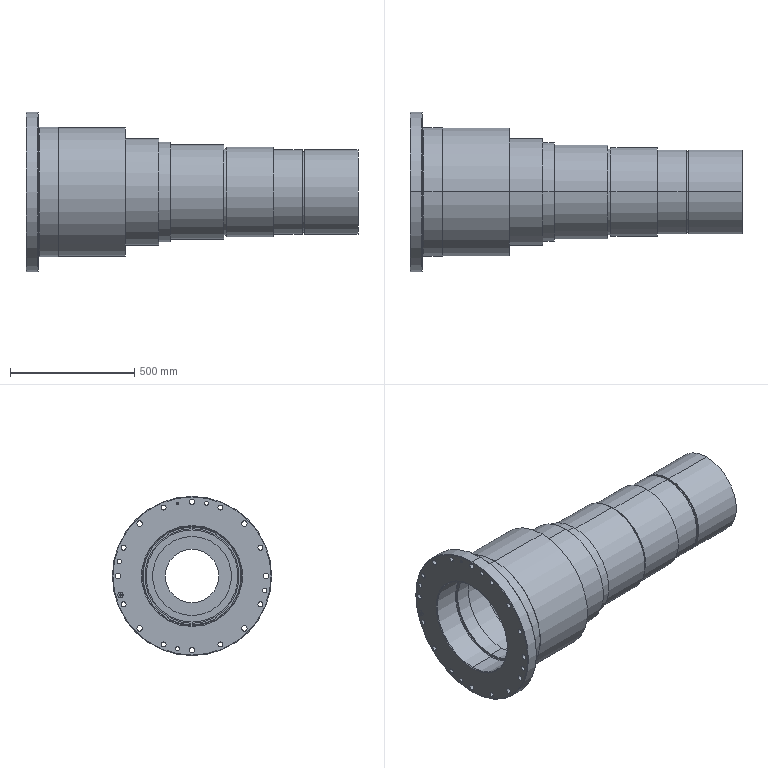Part | SolidWorks | features 3DProfileFeature 2, HoleWzd 2, ICE 2, Revolution 1 | 1 solid | 121 faces | box 1335 x 640 x 640 mm | volume 106671077 mm3 | cylinder 84 | plane 19 | cone 10 | torus 8 | commonest cylinder face diameters 20 x16 22 x16 17.5 x8 340 x4 380 x4 400 x4